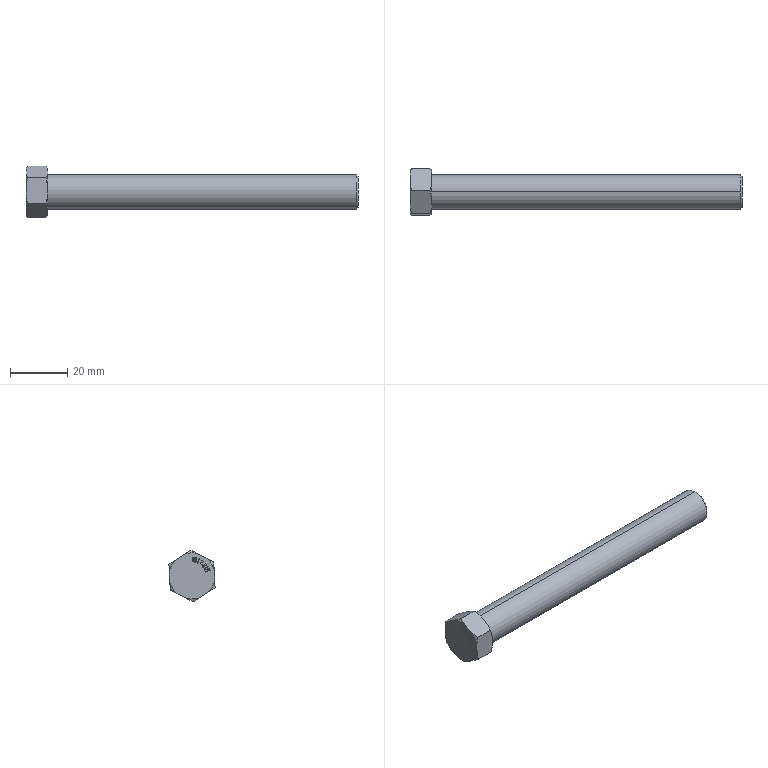Part | SolidWorks | features ICE 2, Chamfer 1, Extrusion 1, MirrorPattern 1, RevCut 1 | 1 solid | 143 faces | box 115.5 x 16.057 x 18 mm | volume 13788 mm3 | plane 75 | spline 50 | cone 16 | cylinder 2 | commonest cylinder face diameters 12 x2